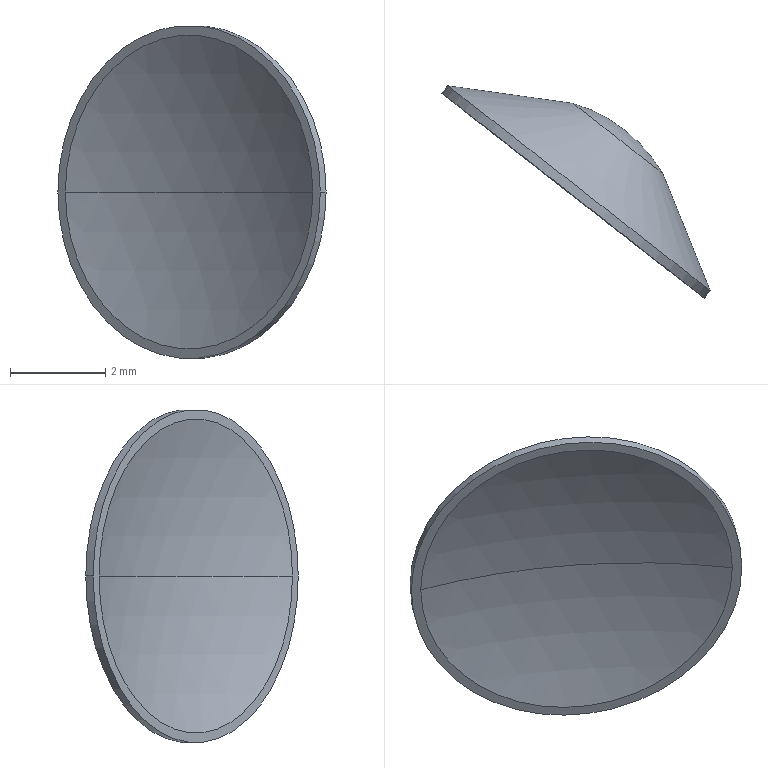Part | STEP file | VALVE_5PARTV11 | 1 solid | 9 faces | box 5.639 x 4.467 x 7 mm | volume 24.483 mm3 | sphere 4 | cone 2 | cylinder 2 | plane 1 | commonest cylinder face diameters 7 x2
STEP:
#1=CARTESIAN_POINT('',(0.,0.,0.));
#2=DIRECTION('',(0.,0.,1.));
#3=DIRECTION('',(1.,0.,0.));
#4=AXIS2_PLACEMENT_3D('',#1,#2,#3);
#5=CARTESIAN_POINT('',(1.825,0.3864,0.));
#6=VERTEX_POINT('',#5);
#7=CARTESIAN_POINT('',(-0.06651,1.864,0.));
#8=VERTEX_POINT('',#7);
#9=CARTESIAN_POINT('',(0.8791,1.125,0.));
#10=DIRECTION('',(-0.6157,-0.788,0.));
#11=DIRECTION('',(0.788,-0.6157,0.));
#12=AXIS2_PLACEMENT_3D('',#9,#10,#11);
#13=CIRCLE('',#12,1.2);
#14=CARTESIAN_POINT('',(0.8791,1.125,0.));
#15=DIRECTION('',(-0.6157,-0.788,0.));
#16=DIRECTION('',(0.788,-0.6157,0.));
#17=AXIS2_PLACEMENT_3D('',#14,#15,#16);
#18=CONICAL_SURFACE('',#17,1.2,1.047);
#19=CARTESIAN_POINT('',(0.,0.));
#20=DIRECTION('',(1.,0.));
#21=VECTOR('',#20,1.);
#22=LINE('',#19,#21);
#23=(GEOMETRIC_REPRESENTATION_CONTEXT(2)PARAMETRIC_REPRESENTATION_CONTEXT()REPRESENTATION_CONTEXT('',''));
#24=DEFINITIONAL_REPRESENTATION('',(#22),#23);
#25=PCURVE('',#18,#24);
#26=CARTESIAN_POINT('',(-0.9763,-1.25,0.));
#27=DIRECTION('',(0.,0.,1.));
#28=DIRECTION('',(0.788,-0.6157,0.));
#29=AXIS2_PLACEMENT_3D('',#26,#27,#28);
#30=SPHERICAL_SURFACE('',#29,3.244);
#31=CARTESIAN_POINT('',(1.192,0.));
#32=CARTESIAN_POINT('',(1.192,0.01761));
#33=CARTESIAN_POINT('',(1.194,0.05283));
#34=CARTESIAN_POINT('',(1.205,0.1047));
#35=CARTESIAN_POINT('',(1.222,0.1548));
#36=CARTESIAN_POINT('',(1.246,0.202));
#37=CARTESIAN_POINT('',(1.277,0.2455));
#38=CARTESIAN_POINT('',(1.315,0.2843));
#39=CARTESIAN_POINT('',(1.358,0.3175));
#40=CARTESIAN_POINT('',(1.406,0.3444));
#41=CARTESIAN_POINT('',(1.459,0.3641));
#42=CARTESIAN_POINT('',(1.514,0.3762));
#43=CARTESIAN_POINT('',(1.571,0.3803));
#44=CARTESIAN_POINT('',(1.628,0.3762));
#45=CARTESIAN_POINT('',(1.683,0.3641));
#46=CARTESIAN_POINT('',(1.735,0.3444));
#47=CARTESIAN_POINT('',(1.784,0.3175));
#48=CARTESIAN_POINT('',(1.827,0.2843));
#49=CARTESIAN_POINT('',(1.864,0.2455));
#50=CARTESIAN_POINT('',(1.895,0.202));
#51=CARTESIAN_POINT('',(1.919,0.1548));
#52=CARTESIAN_POINT('',(1.937,0.1047));
#53=CARTESIAN_POINT('',(1.947,0.05283));
#54=CARTESIAN_POINT('',(1.95,0.01761));
#55=CARTESIAN_POINT('',(1.95,0.));
#56=B_SPLINE_CURVE_WITH_KNOTS('',3,(#31,#32,#33,#34,#35,#36,#37,#38,#39,#40,#41,#42,#43,#44,#45,#46,#47,#48,#49,#50,#51,#52,#53,#54,#55),.UNSPECIFIED.,.F.,.F.,(4,1,1,1,1,1,1,1,1,1,1,1,1,1,1,1,1,1,1,1,1,1,4),(0.,0.1428,0.2856,0.4284,0.5712,0.714,0.8568,0.9996,1.142,1.285,1.428,1.571,1.714,1.856,1.999,2.142,2.285,2.428,2.57,2.713,2.856,2.999,3.142),.QUASI_UNIFORM_KNOTS.);
#57=(GEOMETRIC_REPRESENTATION_CONTEXT(2)PARAMETRIC_REPRESENTATION_CONTEXT()REPRESENTATION_CONTEXT('',''));
#58=DEFINITIONAL_REPRESENTATION('',(#56),#57);
#59=PCURVE('',#30,#58);
#60=SURFACE_CURVE('',#13,(#25,#59),.PCURVE_S1.);
#61=EDGE_CURVE('',#6,#8,#60,.T.);
#62=ORIENTED_EDGE('',*,*,#61,.T.);
#63=CARTESIAN_POINT('',(-2.696,2.234,0.));
#64=VERTEX_POINT('',#63);
#65=CARTESIAN_POINT('',(-0.06651,1.864,0.));
#66=DIRECTION('',(-0.9903,0.1392,0.));
#67=VECTOR('',#66,1.);
#68=LINE('',#65,#67);
#69=CARTESIAN_POINT('',(3.142,0.));
#70=DIRECTION('',(0.,1.));
#71=VECTOR('',#70,1.);
#72=LINE('',#69,#71);
#73=(GEOMETRIC_REPRESENTATION_CONTEXT(2)PARAMETRIC_REPRESENTATION_CONTEXT()REPRESENTATION_CONTEXT('',''));
#74=DEFINITIONAL_REPRESENTATION('',(#72),#73);
#75=PCURVE('',#18,#74);
#76=CARTESIAN_POINT('',(0.8791,1.125,0.));
#77=DIRECTION('',(-0.6157,-0.788,0.));
#78=DIRECTION('',(0.788,-0.6157,0.));
#79=AXIS2_PLACEMENT_3D('',#76,#77,#78);
#80=CONICAL_SURFACE('',#79,1.2,1.047);
#81=CARTESIAN_POINT('',(3.142,0.));
#82=DIRECTION('',(0.,1.));
#83=VECTOR('',#82,1.);
#84=LINE('',#81,#83);
#85=(GEOMETRIC_REPRESENTATION_CONTEXT(2)PARAMETRIC_REPRESENTATION_CONTEXT()REPRESENTATION_CONTEXT('',''));
#86=DEFINITIONAL_REPRESENTATION('',(#84),#85);
#87=PCURVE('',#80,#86);
#88=SURFACE_CURVE('',#68,(#75,#87),.PCURVE_S1.);
#89=EDGE_CURVE('',#8,#64,#88,.T.);
#90=ORIENTED_EDGE('',*,*,#89,.T.);
#91=CARTESIAN_POINT('',(2.82,-2.076,0.));
#92=VERTEX_POINT('',#91);
#93=CARTESIAN_POINT('',(0.06157,0.0788,0.));
#94=DIRECTION('',(-0.6157,-0.788,0.));
#95=DIRECTION('',(0.788,-0.6157,0.));
#96=AXIS2_PLACEMENT_3D('',#93,#94,#95);
#97=CIRCLE('',#96,3.5);
#98=CARTESIAN_POINT('',(0.,1.328));
#99=DIRECTION('',(1.,0.));
#100=VECTOR('',#99,1.);
#101=LINE('',#98,#100);
#102=(GEOMETRIC_REPRESENTATION_CONTEXT(2)PARAMETRIC_REPRESENTATION_CONTEXT()REPRESENTATION_CONTEXT('',''));
#103=DEFINITIONAL_REPRESENTATION('',(#101),#102);
#104=PCURVE('',#18,#103);
#105=CARTESIAN_POINT('',(0.2463,0.3152,0.));
#106=DIRECTION('',(-0.6157,-0.788,0.));
#107=DIRECTION('',(0.788,-0.6157,0.));
#108=AXIS2_PLACEMENT_3D('',#105,#106,#107);
#109=CYLINDRICAL_SURFACE('',#108,3.5);
#110=CARTESIAN_POINT('',(0.,0.3));
#111=DIRECTION('',(1.,0.));
#112=VECTOR('',#111,1.);
#113=LINE('',#110,#112);
#114=(GEOMETRIC_REPRESENTATION_CONTEXT(2)PARAMETRIC_REPRESENTATION_CONTEXT()REPRESENTATION_CONTEXT('',''));
#115=DEFINITIONAL_REPRESENTATION('',(#113),#114);
#116=PCURVE('',#109,#115);
#117=SURFACE_CURVE('',#97,(#104,#116),.PCURVE_S1.);
#118=EDGE_CURVE('',#92,#64,#117,.T.);
#119=ORIENTED_EDGE('',*,*,#118,.F.);
#120=CARTESIAN_POINT('',(1.825,0.3864,0.));
#121=DIRECTION('',(0.3746,-0.9272,0.));
#122=VECTOR('',#121,1.);
#123=LINE('',#120,#122);
#124=CARTESIAN_POINT('',(0.,0.));
#125=DIRECTION('',(0.,1.));
#126=VECTOR('',#125,1.);
#127=LINE('',#124,#126);
#128=(GEOMETRIC_REPRESENTATION_CONTEXT(2)PARAMETRIC_REPRESENTATION_CONTEXT()REPRESENTATION_CONTEXT('',''));
#129=DEFINITIONAL_REPRESENTATION('',(#127),#128);
#130=PCURVE('',#18,#129);
#131=CARTESIAN_POINT('',(6.283,0.));
#132=DIRECTION('',(0.,1.));
#133=VECTOR('',#132,1.);
#134=LINE('',#131,#133);
#135=(GEOMETRIC_REPRESENTATION_CONTEXT(2)PARAMETRIC_REPRESENTATION_CONTEXT()REPRESENTATION_CONTEXT('',''));
#136=DEFINITIONAL_REPRESENTATION('',(#134),#135);
#137=PCURVE('',#80,#136);
#138=SURFACE_CURVE('',#123,(#130,#137),.PCURVE_S1.);
#139=EDGE_CURVE('',#6,#92,#138,.T.);
#140=ORIENTED_EDGE('',*,*,#139,.F.);
#141=EDGE_LOOP('',(#62,#90,#119,#140));
#142=FACE_BOUND('',#141,.T.);
#143=ADVANCED_FACE('',(#142),#18,.T.);
#144=CARTESIAN_POINT('',(1.021,1.307,0.));
#145=VERTEX_POINT('',#144);
#146=CARTESIAN_POINT('',(-0.9763,-1.25,0.));
#147=DIRECTION('',(0.,0.,-1.));
#148=DIRECTION('',(-1.,0.,0.));
#149=AXIS2_PLACEMENT_3D('',#146,#147,#148);
#150=CIRCLE('',#149,3.244);
#151=CARTESIAN_POINT('',(3.805,0.));
#152=DIRECTION('',(-1.,0.));
#153=VECTOR('',#152,1.);
#154=LINE('',#151,#153);
#155=(GEOMETRIC_REPRESENTATION_CONTEXT(2)PARAMETRIC_REPRESENTATION_CONTEXT()REPRESENTATION_CONTEXT('',''));
#156=DEFINITIONAL_REPRESENTATION('',(#154),#155);
#157=PCURVE('',#30,#156);
#158=CARTESIAN_POINT('',(-0.9763,-1.25,0.));
#159=DIRECTION('',(0.,0.,1.));
#160=DIRECTION('',(0.788,-0.6157,0.));
#161=AXIS2_PLACEMENT_3D('',#158,#159,#160);
#162=SPHERICAL_SURFACE('',#161,3.244);
#163=CARTESIAN_POINT('',(3.805,0.));
#164=DIRECTION('',(-1.,0.));
#165=VECTOR('',#164,1.);
#166=LINE('',#163,#165);
#167=(GEOMETRIC_REPRESENTATION_CONTEXT(2)PARAMETRIC_REPRESENTATION_CONTEXT()REPRESENTATION_CONTEXT('',''));
#168=DEFINITIONAL_REPRESENTATION('',(#166),#167);
#169=PCURVE('',#162,#168);
#170=SURFACE_CURVE('',#150,(#157,#169),.PCURVE_S1.);
#171=EDGE_CURVE('',#145,#6,#170,.T.);
#172=ORIENTED_EDGE('',*,*,#171,.F.);
#173=CARTESIAN_POINT('',(-0.9763,-1.25,0.));
#174=DIRECTION('',(0.,0.,1.));
#175=DIRECTION('',(1.,0.,0.));
#176=AXIS2_PLACEMENT_3D('',#173,#174,#175);
#177=CIRCLE('',#176,3.244);
#178=CARTESIAN_POINT('',(0.6632,0.));
#179=DIRECTION('',(1.,0.));
#180=VECTOR('',#179,1.);
#181=LINE('',#178,#180);
#182=(GEOMETRIC_REPRESENTATION_CONTEXT(2)PARAMETRIC_REPRESENTATION_CONTEXT()REPRESENTATION_CONTEXT('',''));
#183=DEFINITIONAL_REPRESENTATION('',(#181),#182);
#184=PCURVE('',#30,#183);
#185=CARTESIAN_POINT('',(0.6632,0.));
#186=DIRECTION('',(1.,0.));
#187=VECTOR('',#186,1.);
#188=LINE('',#185,#187);
#189=(GEOMETRIC_REPRESENTATION_CONTEXT(2)PARAMETRIC_REPRESENTATION_CONTEXT()REPRESENTATION_CONTEXT('',''));
#190=DEFINITIONAL_REPRESENTATION('',(#188),#189);
#191=PCURVE('',#162,#190);
#192=SURFACE_CURVE('',#177,(#184,#191),.PCURVE_S1.);
#193=EDGE_CURVE('',#145,#8,#192,.T.);
#194=ORIENTED_EDGE('',*,*,#193,.T.);
#195=ORIENTED_EDGE('',*,*,#61,.F.);
#196=EDGE_LOOP('',(#172,#194,#195));
#197=FACE_BOUND('',#196,.T.);
#198=ADVANCED_FACE('',(#197),#30,.T.);
#199=CARTESIAN_POINT('',(2.539,-2.11,0.));
#200=VERTEX_POINT('',#199);
#201=CARTESIAN_POINT('',(-2.662,1.953,0.));
#202=VERTEX_POINT('',#201);
#203=CARTESIAN_POINT('',(-0.06157,-0.0788,0.));
#204=DIRECTION('',(-0.6157,-0.788,0.));
#205=DIRECTION('',(0.788,-0.6157,0.));
#206=AXIS2_PLACEMENT_3D('',#203,#204,#205);
#207=CIRCLE('',#206,3.3);
#208=CARTESIAN_POINT('',(-6.612,-8.463,0.));
#209=DIRECTION('',(0.,0.,-1.));
#210=DIRECTION('',(-0.788,0.6157,0.));
#211=AXIS2_PLACEMENT_3D('',#208,#209,#210);
#212=SPHERICAL_SURFACE('',#211,11.14);
#213=CARTESIAN_POINT('',(1.872,0.));
#214=CARTESIAN_POINT('',(1.872,-0.0141));
#215=CARTESIAN_POINT('',(1.87,-0.0423));
#216=CARTESIAN_POINT('',(1.861,-0.08382));
#217=CARTESIAN_POINT('',(1.847,-0.1238));
#218=CARTESIAN_POINT('',(1.827,-0.1614));
#219=CARTESIAN_POINT('',(1.802,-0.1959));
#220=CARTESIAN_POINT('',(1.772,-0.2265));
#221=CARTESIAN_POINT('',(1.738,-0.2527));
#222=CARTESIAN_POINT('',(1.699,-0.2738));
#223=CARTESIAN_POINT('',(1.658,-0.2892));
#224=CARTESIAN_POINT('',(1.615,-0.2986));
#225=CARTESIAN_POINT('',(1.571,-0.3018));
#226=CARTESIAN_POINT('',(1.527,-0.2986));
#227=CARTESIAN_POINT('',(1.483,-0.2892));
#228=CARTESIAN_POINT('',(1.442,-0.2738));
#229=CARTESIAN_POINT('',(1.404,-0.2527));
#230=CARTESIAN_POINT('',(1.37,-0.2265));
#231=CARTESIAN_POINT('',(1.34,-0.1959));
#232=CARTESIAN_POINT('',(1.315,-0.1614));
#233=CARTESIAN_POINT('',(1.295,-0.1238));
#234=CARTESIAN_POINT('',(1.281,-0.08382));
#235=CARTESIAN_POINT('',(1.272,-0.0423));
#236=CARTESIAN_POINT('',(1.27,-0.0141));
#237=CARTESIAN_POINT('',(1.27,0.));
#238=B_SPLINE_CURVE_WITH_KNOTS('',3,(#213,#214,#215,#216,#217,#218,#219,#220,#221,#222,#223,#224,#225,#226,#227,#228,#229,#230,#231,#232,#233,#234,#235,#236,#237),.UNSPECIFIED.,.F.,.F.,(4,1,1,1,1,1,1,1,1,1,1,1,1,1,1,1,1,1,1,1,1,1,4),(0.,0.1428,0.2856,0.4284,0.5712,0.714,0.8568,0.9996,1.142,1.285,1.428,1.571,1.714,1.856,1.999,2.142,2.285,2.428,2.57,2.713,2.856,2.999,3.142),.QUASI_UNIFORM_KNOTS.);
#239=(GEOMETRIC_REPRESENTATION_CONTEXT(2)PARAMETRIC_REPRESENTATION_CONTEXT()REPRESENTATION_CONTEXT('',''));
#240=DEFINITIONAL_REPRESENTATION('',(#238),#239);
#241=PCURVE('',#212,#240);
#242=CARTESIAN_POINT('',(-2.82,2.076,0.));
#243=DIRECTION('',(0.6157,0.788,0.));
#244=DIRECTION('',(-0.788,0.6157,0.));
#245=AXIS2_PLACEMENT_3D('',#242,#243,#244);
#246=PLANE('',#245);
#247=CARTESIAN_POINT('',(-6.8,0.));
#248=CARTESIAN_POINT('',(-6.8,5.716));
#249=CARTESIAN_POINT('',(-1.85,2.858));
#250=CARTESIAN_POINT('',(3.1,0.));
#251=CARTESIAN_POINT('',(-1.85,-2.858));
#252=CARTESIAN_POINT('',(-6.8,-5.716));
#253=CARTESIAN_POINT('',(-6.8,0.));
#254=(BOUNDED_CURVE()B_SPLINE_CURVE(2,(#247,#248,#249,#250,#251,#252,#253),.UNSPECIFIED.,.T.,.F.)B_SPLINE_CURVE_WITH_KNOTS((1,2,2,2,2,1),(-2.094,0.,2.094,4.189,6.283,8.378),.UNSPECIFIED.)CURVE()GEOMETRIC_REPRESENTATION_ITEM()RATIONAL_B_SPLINE_CURVE((1.,0.5,1.,0.5,1.,0.5,1.))REPRESENTATION_ITEM(''));
#255=(GEOMETRIC_REPRESENTATION_CONTEXT(2)PARAMETRIC_REPRESENTATION_CONTEXT()REPRESENTATION_CONTEXT('',''));
#256=DEFINITIONAL_REPRESENTATION('',(#254),#255);
#257=PCURVE('',#246,#256);
#258=SURFACE_CURVE('',#207,(#241,#257),.PCURVE_S1.);
#259=EDGE_CURVE('',#200,#202,#258,.T.);
#260=ORIENTED_EDGE('',*,*,#259,.F.);
#261=CARTESIAN_POINT('',(0.2463,0.3152,0.));
#262=VERTEX_POINT('',#261);
#263=CARTESIAN_POINT('',(-6.612,-8.463,0.));
#264=DIRECTION('',(0.,0.,-1.));
#265=DIRECTION('',(-1.,0.,0.));
#266=AXIS2_PLACEMENT_3D('',#263,#264,#265);
#267=CIRCLE('',#266,11.14);
#268=CARTESIAN_POINT('',(-0.6632,0.));
#269=DIRECTION('',(1.,0.));
#270=VECTOR('',#269,1.);
#271=LINE('',#268,#270);
#272=(GEOMETRIC_REPRESENTATION_CONTEXT(2)PARAMETRIC_REPRESENTATION_CONTEXT()REPRESENTATION_CONTEXT('',''));
#273=DEFINITIONAL_REPRESENTATION('',(#271),#272);
#274=PCURVE('',#212,#273);
#275=CARTESIAN_POINT('',(-6.612,-8.463,0.));
#276=DIRECTION('',(0.,0.,-1.));
#277=DIRECTION('',(-0.788,0.6157,0.));
#278=AXIS2_PLACEMENT_3D('',#275,#276,#277);
#279=SPHERICAL_SURFACE('',#278,11.14);
#280=CARTESIAN_POINT('',(-0.6632,0.));
#281=DIRECTION('',(1.,0.));
#282=VECTOR('',#281,1.);
#283=LINE('',#280,#282);
#284=(GEOMETRIC_REPRESENTATION_CONTEXT(2)PARAMETRIC_REPRESENTATION_CONTEXT()REPRESENTATION_CONTEXT('',''));
#285=DEFINITIONAL_REPRESENTATION('',(#283),#284);
#286=PCURVE('',#279,#285);
#287=SURFACE_CURVE('',#267,(#274,#286),.PCURVE_S1.);
#288=EDGE_CURVE('',#262,#200,#287,.T.);
#289=ORIENTED_EDGE('',*,*,#288,.F.);
#290=CARTESIAN_POINT('',(-6.612,-8.463,0.));
#291=DIRECTION('',(0.,0.,1.));
#292=DIRECTION('',(1.,0.,0.));
#293=AXIS2_PLACEMENT_3D('',#290,#291,#292);
#294=CIRCLE('',#293,11.14);
#295=CARTESIAN_POINT('',(2.478,0.));
#296=DIRECTION('',(-1.,0.));
#297=VECTOR('',#296,1.);
#298=LINE('',#295,#297);
#299=(GEOMETRIC_REPRESENTATION_CONTEXT(2)PARAMETRIC_REPRESENTATION_CONTEXT()REPRESENTATION_CONTEXT('',''));
#300=DEFINITIONAL_REPRESENTATION('',(#298),#299);
#301=PCURVE('',#212,#300);
#302=CARTESIAN_POINT('',(2.478,0.));
#303=DIRECTION('',(-1.,0.));
#304=VECTOR('',#303,1.);
#305=LINE('',#302,#304);
#306=(GEOMETRIC_REPRESENTATION_CONTEXT(2)PARAMETRIC_REPRESENTATION_CONTEXT()REPRESENTATION_CONTEXT('',''));
#307=DEFINITIONAL_REPRESENTATION('',(#305),#306);
#308=PCURVE('',#279,#307);
#309=SURFACE_CURVE('',#294,(#301,#308),.PCURVE_S1.);
#310=EDGE_CURVE('',#262,#202,#309,.T.);
#311=ORIENTED_EDGE('',*,*,#310,.T.);
#312=EDGE_LOOP('',(#260,#289,#311));
#313=FACE_BOUND('',#312,.F.);
#314=ADVANCED_FACE('',(#313),#212,.F.);
#315=ORIENTED_EDGE('',*,*,#118,.T.);
#316=CARTESIAN_POINT('',(-2.82,2.076,0.));
#317=VERTEX_POINT('',#316);
#318=CARTESIAN_POINT('',(-2.512,2.47,0.));
#319=DIRECTION('',(-0.6157,-0.788,0.));
#320=VECTOR('',#319,1.);
#321=LINE('',#318,#320);
#322=CARTESIAN_POINT('',(3.142,0.));
#323=DIRECTION('',(0.,1.));
#324=VECTOR('',#323,1.);
#325=LINE('',#322,#324);
#326=(GEOMETRIC_REPRESENTATION_CONTEXT(2)PARAMETRIC_REPRESENTATION_CONTEXT()REPRESENTATION_CONTEXT('',''));
#327=DEFINITIONAL_REPRESENTATION('',(#325),#326);
#328=PCURVE('',#109,#327);
#329=CARTESIAN_POINT('',(0.2463,0.3152,0.));
#330=DIRECTION('',(-0.6157,-0.788,0.));
#331=DIRECTION('',(0.788,-0.6157,0.));
#332=AXIS2_PLACEMENT_3D('',#329,#330,#331);
#333=CYLINDRICAL_SURFACE('',#332,3.5);
#334=CARTESIAN_POINT('',(3.142,0.));
#335=DIRECTION('',(0.,1.));
#336=VECTOR('',#335,1.);
#337=LINE('',#334,#336);
#338=(GEOMETRIC_REPRESENTATION_CONTEXT(2)PARAMETRIC_REPRESENTATION_CONTEXT()REPRESENTATION_CONTEXT('',''));
#339=DEFINITIONAL_REPRESENTATION('',(#337),#338);
#340=PCURVE('',#333,#339);
#341=SURFACE_CURVE('',#321,(#328,#340),.PCURVE_S1.);
#342=EDGE_CURVE('',#64,#317,#341,.T.);
#343=ORIENTED_EDGE('',*,*,#342,.T.);
#344=CARTESIAN_POINT('',(2.696,-2.234,0.));
#345=VERTEX_POINT('',#344);
#346=CARTESIAN_POINT('',(-0.06157,-0.0788,0.));
#347=DIRECTION('',(-0.6157,-0.788,0.));
#348=DIRECTION('',(0.788,-0.6157,0.));
#349=AXIS2_PLACEMENT_3D('',#346,#347,#348);
#350=CIRCLE('',#349,3.5);
#351=CARTESIAN_POINT('',(0.,0.5));
#352=DIRECTION('',(1.,0.));
#353=VECTOR('',#352,1.);
#354=LINE('',#351,#353);
#355=(GEOMETRIC_REPRESENTATION_CONTEXT(2)PARAMETRIC_REPRESENTATION_CONTEXT()REPRESENTATION_CONTEXT('',''));
#356=DEFINITIONAL_REPRESENTATION('',(#354),#355);
#357=PCURVE('',#109,#356);
#358=CARTESIAN_POINT('',(-7.,0.));
#359=CARTESIAN_POINT('',(-7.,6.062));
#360=CARTESIAN_POINT('',(-1.75,3.031));
#361=CARTESIAN_POINT('',(3.5,0.));
#362=CARTESIAN_POINT('',(-1.75,-3.031));
#363=CARTESIAN_POINT('',(-7.,-6.062));
#364=CARTESIAN_POINT('',(-7.,0.));
#365=(BOUNDED_CURVE()B_SPLINE_CURVE(2,(#358,#359,#360,#361,#362,#363,#364),.UNSPECIFIED.,.T.,.F.)B_SPLINE_CURVE_WITH_KNOTS((1,2,2,2,2,1),(-2.094,0.,2.094,4.189,6.283,8.378),.UNSPECIFIED.)CURVE()GEOMETRIC_REPRESENTATION_ITEM()RATIONAL_B_SPLINE_CURVE((1.,0.5,1.,0.5,1.,0.5,1.))REPRESENTATION_ITEM(''));
#366=(GEOMETRIC_REPRESENTATION_CONTEXT(2)PARAMETRIC_REPRESENTATION_CONTEXT()REPRESENTATION_CONTEXT('',''));
#367=DEFINITIONAL_REPRESENTATION('',(#365),#366);
#368=PCURVE('',#246,#367);
#369=SURFACE_CURVE('',#350,(#357,#368),.PCURVE_S1.);
#370=EDGE_CURVE('',#345,#317,#369,.T.);
#371=ORIENTED_EDGE('',*,*,#370,.F.);
#372=CARTESIAN_POINT('',(3.004,-1.84,0.));
#373=DIRECTION('',(-0.6157,-0.788,0.));
#374=VECTOR('',#373,1.);
#375=LINE('',#372,#374);
#376=CARTESIAN_POINT('',(0.,0.));
#377=DIRECTION('',(0.,1.));
#378=VECTOR('',#377,1.);
#379=LINE('',#376,#378);
#380=(GEOMETRIC_REPRESENTATION_CONTEXT(2)PARAMETRIC_REPRESENTATION_CONTEXT()REPRESENTATION_CONTEXT('',''));
#381=DEFINITIONAL_REPRESENTATION('',(#379),#380);
#382=PCURVE('',#109,#381);
#383=CARTESIAN_POINT('',(6.283,0.));
#384=DIRECTION('',(0.,1.));
#385=VECTOR('',#384,1.);
#386=LINE('',#383,#385);
#387=(GEOMETRIC_REPRESENTATION_CONTEXT(2)PARAMETRIC_REPRESENTATION_CONTEXT()REPRESENTATION_CONTEXT('',''));
#388=DEFINITIONAL_REPRESENTATION('',(#386),#387);
#389=PCURVE('',#333,#388);
#390=SURFACE_CURVE('',#375,(#382,#389),.PCURVE_S1.);
#391=EDGE_CURVE('',#92,#345,#390,.T.);
#392=ORIENTED_EDGE('',*,*,#391,.F.);
#393=EDGE_LOOP('',(#315,#343,#371,#392));
#394=FACE_BOUND('',#393,.T.);
#395=ADVANCED_FACE('',(#394),#109,.T.);
#396=ORIENTED_EDGE('',*,*,#342,.F.);
#397=CARTESIAN_POINT('',(0.06157,0.0788,0.));
#398=DIRECTION('',(-0.6157,-0.788,0.));
#399=DIRECTION('',(0.788,-0.6157,0.));
#400=AXIS2_PLACEMENT_3D('',#397,#398,#399);
#401=CIRCLE('',#400,3.5);
#402=CARTESIAN_POINT('',(0.,0.3));
#403=DIRECTION('',(1.,0.));
#404=VECTOR('',#403,1.);
#405=LINE('',#402,#404);
#406=(GEOMETRIC_REPRESENTATION_CONTEXT(2)PARAMETRIC_REPRESENTATION_CONTEXT()REPRESENTATION_CONTEXT('',''));
#407=DEFINITIONAL_REPRESENTATION('',(#405),#406);
#408=PCURVE('',#333,#407);
#409=CARTESIAN_POINT('',(0.,1.328));
#410=DIRECTION('',(1.,0.));
#411=VECTOR('',#410,1.);
#412=LINE('',#409,#411);
#413=(GEOMETRIC_REPRESENTATION_CONTEXT(2)PARAMETRIC_REPRESENTATION_CONTEXT()REPRESENTATION_CONTEXT('',''));
#414=DEFINITIONAL_REPRESENTATION('',(#412),#413);
#415=PCURVE('',#80,#414);
#416=SURFACE_CURVE('',#401,(#408,#415),.PCURVE_S1.);
#417=EDGE_CURVE('',#64,#92,#416,.T.);
#418=ORIENTED_EDGE('',*,*,#417,.T.);
#419=ORIENTED_EDGE('',*,*,#391,.T.);
#420=CARTESIAN_POINT('',(-0.06157,-0.0788,0.));
#421=DIRECTION('',(-0.6157,-0.788,0.));
#422=DIRECTION('',(0.788,-0.6157,0.));
#423=AXIS2_PLACEMENT_3D('',#420,#421,#422);
#424=CIRCLE('',#423,3.5);
#425=CARTESIAN_POINT('',(0.,0.5));
#426=DIRECTION('',(1.,0.));
#427=VECTOR('',#426,1.);
#428=LINE('',#425,#427);
#429=(GEOMETRIC_REPRESENTATION_CONTEXT(2)PARAMETRIC_REPRESENTATION_CONTEXT()REPRESENTATION_CONTEXT('',''));
#430=DEFINITIONAL_REPRESENTATION('',(#428),#429);
#431=PCURVE('',#333,#430);
#432=CARTESIAN_POINT('',(-7.,0.));
#433=CARTESIAN_POINT('',(-7.,6.062));
#434=CARTESIAN_POINT('',(-1.75,3.031));
#435=CARTESIAN_POINT('',(3.5,0.));
#436=CARTESIAN_POINT('',(-1.75,-3.031));
#437=CARTESIAN_POINT('',(-7.,-6.062));
#438=CARTESIAN_POINT('',(-7.,0.));
#439=(BOUNDED_CURVE()B_SPLINE_CURVE(2,(#432,#433,#434,#435,#436,#437,#438),.UNSPECIFIED.,.T.,.F.)B_SPLINE_CURVE_WITH_KNOTS((1,2,2,2,2,1),(-2.094,0.,2.094,4.189,6.283,8.378),.UNSPECIFIED.)CURVE()GEOMETRIC_REPRESENTATION_ITEM()RATIONAL_B_SPLINE_CURVE((1.,0.5,1.,0.5,1.,0.5,1.))REPRESENTATION_ITEM(''));
#440=(GEOMETRIC_REPRESENTATION_CONTEXT(2)PARAMETRIC_REPRESENTATION_CONTEXT()REPRESENTATION_CONTEXT('',''));
#441=DEFINITIONAL_REPRESENTATION('',(#439),#440);
#442=PCURVE('',#246,#441);
#443=SURFACE_CURVE('',#424,(#431,#442),.PCURVE_S1.);
#444=EDGE_CURVE('',#317,#345,#443,.T.);
#445=ORIENTED_EDGE('',*,*,#444,.F.);
#446=EDGE_LOOP('',(#396,#418,#419,#445));
#447=FACE_BOUND('',#446,.T.);
#448=ADVANCED_FACE('',(#447),#333,.T.);
#449=CARTESIAN_POINT('',(-0.06157,-0.0788,0.));
#450=DIRECTION('',(-0.6157,-0.788,0.));
#451=DIRECTION('',(0.788,-0.6157,0.));
#452=AXIS2_PLACEMENT_3D('',#449,#450,#451);
#453=CIRCLE('',#452,3.3);
#454=CARTESIAN_POINT('',(-6.8,0.));
#455=CARTESIAN_POINT('',(-6.8,5.716));
#456=CARTESIAN_POINT('',(-1.85,2.858));
#457=CARTESIAN_POINT('',(3.1,0.));
#458=CARTESIAN_POINT('',(-1.85,-2.858));
#459=CARTESIAN_POINT('',(-6.8,-5.716));
#460=CARTESIAN_POINT('',(-6.8,0.));
#461=(BOUNDED_CURVE()B_SPLINE_CURVE(2,(#454,#455,#456,#457,#458,#459,#460),.UNSPECIFIED.,.T.,.F.)B_SPLINE_CURVE_WITH_KNOTS((1,2,2,2,2,1),(-2.094,0.,2.094,4.189,6.283,8.378),.UNSPECIFIED.)CURVE()GEOMETRIC_REPRESENTATION_ITEM()RATIONAL_B_SPLINE_CURVE((1.,0.5,1.,0.5,1.,0.5,1.))REPRESENTATION_ITEM(''));
#462=(GEOMETRIC_REPRESENTATION_CONTEXT(2)PARAMETRIC_REPRESENTATION_CONTEXT()REPRESENTATION_CONTEXT('',''));
#463=DEFINITIONAL_REPRESENTATION('',(#461),#462);
#464=PCURVE('',#246,#463);
#465=CARTESIAN_POINT('',(1.27,0.));
#466=CARTESIAN_POINT('',(1.27,0.0141));
#467=CARTESIAN_POINT('',(1.272,0.0423));
#468=CARTESIAN_POINT('',(1.281,0.08382));
#469=CARTESIAN_POINT('',(1.295,0.1238));
#470=CARTESIAN_POINT('',(1.315,0.1614));
#471=CARTESIAN_POINT('',(1.34,0.1959));
#472=CARTESIAN_POINT('',(1.37,0.2265));
#473=CARTESIAN_POINT('',(1.404,0.2527));
#474=CARTESIAN_POINT('',(1.442,0.2738));
#475=CARTESIAN_POINT('',(1.483,0.2892));
#476=CARTESIAN_POINT('',(1.527,0.2986));
#477=CARTESIAN_POINT('',(1.571,0.3018));
#478=CARTESIAN_POINT('',(1.615,0.2986));
#479=CARTESIAN_POINT('',(1.658,0.2892));
#480=CARTESIAN_POINT('',(1.699,0.2738));
#481=CARTESIAN_POINT('',(1.738,0.2527));
#482=CARTESIAN_POINT('',(1.772,0.2265));
#483=CARTESIAN_POINT('',(1.802,0.1959));
#484=CARTESIAN_POINT('',(1.827,0.1614));
#485=CARTESIAN_POINT('',(1.847,0.1238));
#486=CARTESIAN_POINT('',(1.861,0.08382));
#487=CARTESIAN_POINT('',(1.87,0.0423));
#488=CARTESIAN_POINT('',(1.872,0.0141));
#489=CARTESIAN_POINT('',(1.872,0.));
#490=B_SPLINE_CURVE_WITH_KNOTS('',3,(#465,#466,#467,#468,#469,#470,#471,#472,#473,#474,#475,#476,#477,#478,#479,#480,#481,#482,#483,#484,#485,#486,#487,#488,#489),.UNSPECIFIED.,.F.,.F.,(4,1,1,1,1,1,1,1,1,1,1,1,1,1,1,1,1,1,1,1,1,1,4),(3.142,3.284,3.427,3.57,3.713,3.856,3.998,4.141,4.284,4.427,4.57,4.712,4.855,4.998,5.141,5.284,5.426,5.569,5.712,5.855,5.998,6.14,6.283),.QUASI_UNIFORM_KNOTS.);
#491=(GEOMETRIC_REPRESENTATION_CONTEXT(2)PARAMETRIC_REPRESENTATION_CONTEXT()REPRESENTATION_CONTEXT('',''));
#492=DEFINITIONAL_REPRESENTATION('',(#490),#491);
#493=PCURVE('',#279,#492);
#494=SURFACE_CURVE('',#453,(#464,#493),.PCURVE_S1.);
#495=EDGE_CURVE('',#202,#200,#494,.T.);
#496=ORIENTED_EDGE('',*,*,#495,.F.);
#497=ORIENTED_EDGE('',*,*,#259,.F.);
#498=EDGE_LOOP('',(#496,#497));
#499=FACE_BOUND('',#498,.T.);
#500=ORIENTED_EDGE('',*,*,#370,.T.);
#501=ORIENTED_EDGE('',*,*,#444,.T.);
#502=EDGE_LOOP('',(#500,#501));
#503=FACE_BOUND('',#502,.T.);
#504=ADVANCED_FACE('',(#499,#503),#246,.F.);
#505=ORIENTED_EDGE('',*,*,#495,.F.);
#506=ORIENTED_EDGE('',*,*,#310,.F.);
#507=ORIENTED_EDGE('',*,*,#288,.T.);
#508=EDGE_LOOP('',(#505,#506,#507));
#509=FACE_BOUND('',#508,.F.);
#510=ADVANCED_FACE('',(#509),#279,.F.);
#511=ORIENTED_EDGE('',*,*,#193,.F.);
#512=ORIENTED_EDGE('',*,*,#171,.T.);
#513=CARTESIAN_POINT('',(0.8791,1.125,0.));
#514=DIRECTION('',(-0.6157,-0.788,0.));
#515=DIRECTION('',(0.788,-0.6157,0.));
#516=AXIS2_PLACEMENT_3D('',#513,#514,#515);
#517=CIRCLE('',#516,1.2);
#518=CARTESIAN_POINT('',(1.95,0.));
#519=CARTESIAN_POINT('',(1.95,-0.01761));
#520=CARTESIAN_POINT('',(1.947,-0.05283));
#521=CARTESIAN_POINT('',(1.937,-0.1047));
#522=CARTESIAN_POINT('',(1.919,-0.1548));
#523=CARTESIAN_POINT('',(1.895,-0.202));
#524=CARTESIAN_POINT('',(1.864,-0.2455));
#525=CARTESIAN_POINT('',(1.827,-0.2843));
#526=CARTESIAN_POINT('',(1.784,-0.3175));
#527=CARTESIAN_POINT('',(1.735,-0.3444));
#528=CARTESIAN_POINT('',(1.683,-0.3641));
#529=CARTESIAN_POINT('',(1.628,-0.3762));
#530=CARTESIAN_POINT('',(1.571,-0.3803));
#531=CARTESIAN_POINT('',(1.514,-0.3762));
#532=CARTESIAN_POINT('',(1.459,-0.3641));
#533=CARTESIAN_POINT('',(1.406,-0.3444));
#534=CARTESIAN_POINT('',(1.358,-0.3175));
#535=CARTESIAN_POINT('',(1.315,-0.2843));
#536=CARTESIAN_POINT('',(1.277,-0.2455));
#537=CARTESIAN_POINT('',(1.246,-0.202));
#538=CARTESIAN_POINT('',(1.222,-0.1548));
#539=CARTESIAN_POINT('',(1.205,-0.1047));
#540=CARTESIAN_POINT('',(1.194,-0.05283));
#541=CARTESIAN_POINT('',(1.192,-0.01761));
#542=CARTESIAN_POINT('',(1.192,0.));
#543=B_SPLINE_CURVE_WITH_KNOTS('',3,(#518,#519,#520,#521,#522,#523,#524,#525,#526,#527,#528,#529,#530,#531,#532,#533,#534,#535,#536,#537,#538,#539,#540,#541,#542),.UNSPECIFIED.,.F.,.F.,(4,1,1,1,1,1,1,1,1,1,1,1,1,1,1,1,1,1,1,1,1,1,4),(3.142,3.284,3.427,3.57,3.713,3.856,3.998,4.141,4.284,4.427,4.57,4.712,4.855,4.998,5.141,5.284,5.426,5.569,5.712,5.855,5.998,6.14,6.283),.QUASI_UNIFORM_KNOTS.);
#544=(GEOMETRIC_REPRESENTATION_CONTEXT(2)PARAMETRIC_REPRESENTATION_CONTEXT()REPRESENTATION_CONTEXT('',''));
#545=DEFINITIONAL_REPRESENTATION('',(#543),#544);
#546=PCURVE('',#162,#545);
#547=CARTESIAN_POINT('',(0.,0.));
#548=DIRECTION('',(1.,0.));
#549=VECTOR('',#548,1.);
#550=LINE('',#547,#549);
#551=(GEOMETRIC_REPRESENTATION_CONTEXT(2)PARAMETRIC_REPRESENTATION_CONTEXT()REPRESENTATION_CONTEXT('',''));
#552=DEFINITIONAL_REPRESENTATION('',(#550),#551);
#553=PCURVE('',#80,#552);
#554=SURFACE_CURVE('',#517,(#546,#553),.PCURVE_S1.);
#555=EDGE_CURVE('',#8,#6,#554,.T.);
#556=ORIENTED_EDGE('',*,*,#555,.F.);
#557=EDGE_LOOP('',(#511,#512,#556));
#558=FACE_BOUND('',#557,.T.);
#559=ADVANCED_FACE('',(#558),#162,.T.);
#560=ORIENTED_EDGE('',*,*,#89,.F.);
#561=ORIENTED_EDGE('',*,*,#555,.T.);
#562=ORIENTED_EDGE('',*,*,#139,.T.);
#563=ORIENTED_EDGE('',*,*,#417,.F.);
#564=EDGE_LOOP('',(#560,#561,#562,#563));
#565=FACE_BOUND('',#564,.T.);
#566=ADVANCED_FACE('',(#565),#80,.T.);
#567=CLOSED_SHELL('',(#143,#198,#314,#395,#448,#504,#510,#559,#566));
#568=MANIFOLD_SOLID_BREP('',#567);
#569=(LENGTH_UNIT()NAMED_UNIT(*)SI_UNIT(.MILLI.,.METRE.));
#570=UNCERTAINTY_MEASURE_WITH_UNIT(LENGTH_MEASURE(0.0000001),#569,'','');
#571=(NAMED_UNIT(*)PLANE_ANGLE_UNIT()SI_UNIT($,.RADIAN.));
#572=(NAMED_UNIT(*)SI_UNIT($,.STERADIAN.)SOLID_ANGLE_UNIT());
#573=(GEOMETRIC_REPRESENTATION_CONTEXT(3)GLOBAL_UNCERTAINTY_ASSIGNED_CONTEXT((#570))GLOBAL_UNIT_ASSIGNED_CONTEXT((#569,#571,#572))REPRESENTATION_CONTEXT('',''));
#574=ADVANCED_BREP_SHAPE_REPRESENTATION('',(#4,#568),#573);